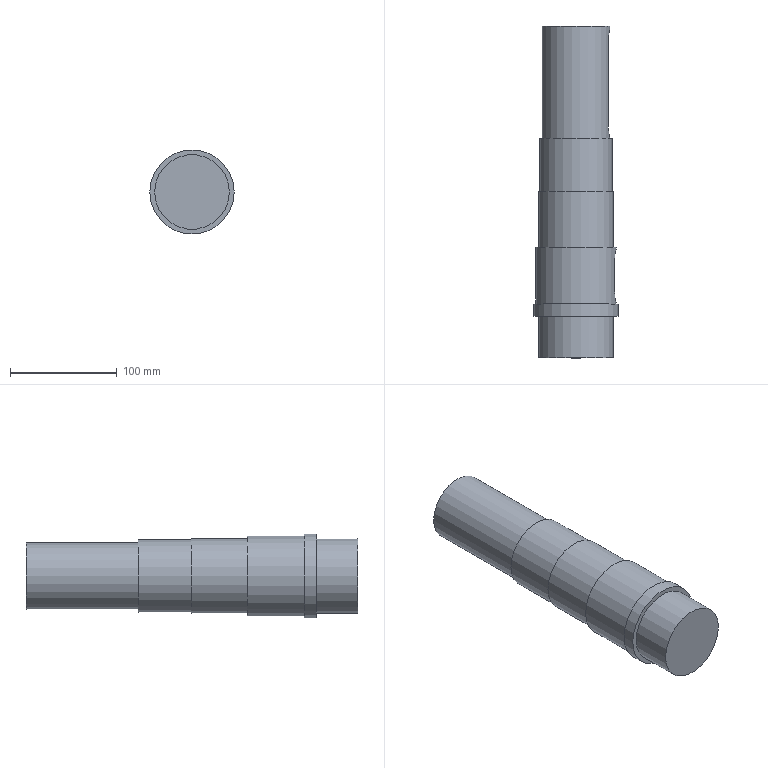Part | NX | features DATUM_CSYS 9, EXTRUDE 8, SKETCH 8, BLEND 2 | 1 solid | 23 faces | box 79 x 311 x 79 mm | volume 1137641 mm3 | plane 13 | cylinder 10 | commonest cylinder face diameters 18 x2 20 x2 70 x2 63 x1 68 x1 75 x1
STEP:
#1=CARTESIAN_POINT('',(35.,0.,0.));
#2=VERTEX_POINT('',#1);
#3=CARTESIAN_POINT('',(0.,0.,0.));
#4=DIRECTION('',(0.,-1.,0.));
#5=DIRECTION('',(1.,0.,0.));
#6=AXIS2_PLACEMENT_3D('',#3,#4,#5);
#7=CIRCLE('',#6,35.);
#8=EDGE_CURVE('',#2,#2,#7,.T.);
#9=ORIENTED_EDGE('',*,*,#8,.T.);
#10=EDGE_LOOP('',(#9));
#11=FACE_BOUND('',#10,.T.);
#12=CARTESIAN_POINT('',(35.,-39.,0.));
#13=VERTEX_POINT('',#12);
#14=CARTESIAN_POINT('',(0.,-39.,0.));
#15=DIRECTION('',(0.,-1.,0.));
#16=DIRECTION('',(1.,0.,0.));
#17=AXIS2_PLACEMENT_3D('',#14,#15,#16);
#18=CIRCLE('',#17,35.);
#19=EDGE_CURVE('',#13,#13,#18,.T.);
#20=ORIENTED_EDGE('',*,*,#19,.F.);
#21=EDGE_LOOP('',(#20));
#22=FACE_BOUND('',#21,.T.);
#23=CARTESIAN_POINT('',(0.,0.,0.));
#24=DIRECTION('',(0.,-1.,0.));
#25=DIRECTION('',(0.,0.,-1.));
#26=AXIS2_PLACEMENT_3D('',#23,#24,#25);
#27=CYLINDRICAL_SURFACE('',#26,35.);
#28=ADVANCED_FACE('',(#11,#22),#27,.T.);
#29=ORIENTED_EDGE('',*,*,#19,.T.);
#30=EDGE_LOOP('',(#29));
#31=FACE_BOUND('',#30,.T.);
#32=CARTESIAN_POINT('',(0.,-39.,0.));
#33=DIRECTION('',(0.,-1.,0.));
#34=DIRECTION('',(0.,0.,-1.));
#35=AXIS2_PLACEMENT_3D('',#32,#33,#34);
#36=PLANE('',#35);
#37=ADVANCED_FACE('',(#31),#36,.T.);
#38=CARTESIAN_POINT('',(39.5,0.,0.));
#39=VERTEX_POINT('',#38);
#40=CARTESIAN_POINT('',(0.,0.,0.));
#41=DIRECTION('',(0.,1.,0.));
#42=DIRECTION('',(1.,0.,0.));
#43=AXIS2_PLACEMENT_3D('',#40,#41,#42);
#44=CIRCLE('',#43,39.5);
#45=EDGE_CURVE('',#39,#39,#44,.T.);
#46=ORIENTED_EDGE('',*,*,#45,.T.);
#47=EDGE_LOOP('',(#46));
#48=FACE_BOUND('',#47,.T.);
#49=CARTESIAN_POINT('',(39.5,11.5,0.));
#50=VERTEX_POINT('',#49);
#51=CARTESIAN_POINT('',(0.,11.5,0.));
#52=DIRECTION('',(0.,1.,0.));
#53=DIRECTION('',(1.,0.,0.));
#54=AXIS2_PLACEMENT_3D('',#51,#52,#53);
#55=CIRCLE('',#54,39.5);
#56=EDGE_CURVE('',#50,#50,#55,.T.);
#57=ORIENTED_EDGE('',*,*,#56,.F.);
#58=EDGE_LOOP('',(#57));
#59=FACE_BOUND('',#58,.T.);
#60=CARTESIAN_POINT('',(0.,0.,0.));
#61=DIRECTION('',(0.,1.,0.));
#62=DIRECTION('',(0.,0.,1.));
#63=AXIS2_PLACEMENT_3D('',#60,#61,#62);
#64=CYLINDRICAL_SURFACE('',#63,39.5);
#65=ADVANCED_FACE('',(#48,#59),#64,.T.);
#66=ORIENTED_EDGE('',*,*,#8,.F.);
#67=EDGE_LOOP('',(#66));
#68=FACE_BOUND('',#67,.T.);
#69=ORIENTED_EDGE('',*,*,#45,.F.);
#70=EDGE_LOOP('',(#69));
#71=FACE_BOUND('',#70,.T.);
#72=CARTESIAN_POINT('',(0.,0.,0.));
#73=DIRECTION('',(0.,1.,0.));
#74=DIRECTION('',(0.,0.,1.));
#75=AXIS2_PLACEMENT_3D('',#72,#73,#74);
#76=PLANE('',#75);
#77=ADVANCED_FACE('',(#68,#71),#76,.F.);
#78=CARTESIAN_POINT('',(37.5,11.5,0.));
#79=VERTEX_POINT('',#78);
#80=CARTESIAN_POINT('',(0.,11.5,0.));
#81=DIRECTION('',(0.,1.,0.));
#82=DIRECTION('',(1.,0.,0.));
#83=AXIS2_PLACEMENT_3D('',#80,#81,#82);
#84=CIRCLE('',#83,37.5);
#85=EDGE_CURVE('',#79,#79,#84,.T.);
#86=ORIENTED_EDGE('',*,*,#85,.F.);
#87=EDGE_LOOP('',(#86));
#88=FACE_BOUND('',#87,.T.);
#89=ORIENTED_EDGE('',*,*,#56,.T.);
#90=EDGE_LOOP('',(#89));
#91=FACE_BOUND('',#90,.T.);
#92=CARTESIAN_POINT('',(0.,11.5,0.));
#93=DIRECTION('',(0.,1.,0.));
#94=DIRECTION('',(0.,0.,1.));
#95=AXIS2_PLACEMENT_3D('',#92,#93,#94);
#96=PLANE('',#95);
#97=ADVANCED_FACE('',(#88,#91),#96,.T.);
#98=CARTESIAN_POINT('',(36.142,23.,-10.));
#99=VERTEX_POINT('',#98);
#100=CARTESIAN_POINT('',(36.142,23.,10.));
#101=VERTEX_POINT('',#100);
#102=CARTESIAN_POINT('',(36.142,23.,-10.));
#103=CARTESIAN_POINT('',(36.142,20.346,-10.));
#104=CARTESIAN_POINT('',(36.649,16.486,-8.359));
#105=CARTESIAN_POINT('',(37.352,13.534,-3.955));
#106=CARTESIAN_POINT('',(37.656,12.461,1.328));
#107=CARTESIAN_POINT('',(36.838,15.18,7.826));
#108=CARTESIAN_POINT('',(36.142,20.346,10.));
#109=CARTESIAN_POINT('',(36.142,23.,10.));
#110=B_SPLINE_CURVE_WITH_KNOTS('',3,(#102,#103,#104,#105,#106,#107,#108,#109),.UNSPECIFIED.,.F.,.F.,(4,1,1,1,1,4),(0.,0.007847,0.01177,0.01569,0.02354,0.03139),.UNSPECIFIED.);
#111=EDGE_CURVE('',#99,#101,#110,.T.);
#112=ORIENTED_EDGE('',*,*,#111,.T.);
#113=CARTESIAN_POINT('',(36.142,53.,10.));
#114=VERTEX_POINT('',#113);
#115=CARTESIAN_POINT('',(36.142,11.5,10.));
#116=DIRECTION('',(0.,1.,0.));
#117=VECTOR('',#116,1000.);
#118=LINE('',#115,#117);
#119=EDGE_CURVE('',#114,#101,#118,.F.);
#120=ORIENTED_EDGE('',*,*,#119,.F.);
#121=CARTESIAN_POINT('',(36.142,53.,-10.));
#122=VERTEX_POINT('',#121);
#123=CARTESIAN_POINT('',(36.142,53.,10.));
#124=CARTESIAN_POINT('',(36.142,55.654,10.));
#125=CARTESIAN_POINT('',(36.649,59.514,8.359));
#126=CARTESIAN_POINT('',(37.352,62.466,3.955));
#127=CARTESIAN_POINT('',(37.656,63.539,-1.328));
#128=CARTESIAN_POINT('',(36.838,60.82,-7.826));
#129=CARTESIAN_POINT('',(36.142,55.654,-10.));
#130=CARTESIAN_POINT('',(36.142,53.,-10.));
#131=B_SPLINE_CURVE_WITH_KNOTS('',3,(#123,#124,#125,#126,#127,#128,#129,#130),.UNSPECIFIED.,.F.,.F.,(4,1,1,1,1,4),(-0.01569,-0.007846,-0.003923,0.000000187,0.007847,0.01569),.UNSPECIFIED.);
#132=EDGE_CURVE('',#114,#122,#131,.T.);
#133=ORIENTED_EDGE('',*,*,#132,.T.);
#134=CARTESIAN_POINT('',(36.142,11.5,-10.));
#135=DIRECTION('',(0.,1.,0.));
#136=VECTOR('',#135,1000.);
#137=LINE('',#134,#136);
#138=EDGE_CURVE('',#99,#122,#137,.T.);
#139=ORIENTED_EDGE('',*,*,#138,.F.);
#140=EDGE_LOOP('',(#112,#120,#133,#139));
#141=FACE_BOUND('',#140,.T.);
#142=ORIENTED_EDGE('',*,*,#85,.T.);
#143=EDGE_LOOP('',(#142));
#144=FACE_BOUND('',#143,.T.);
#145=CARTESIAN_POINT('',(37.5,64.5,0.));
#146=VERTEX_POINT('',#145);
#147=CARTESIAN_POINT('',(0.,64.5,0.));
#148=DIRECTION('',(0.,1.,0.));
#149=DIRECTION('',(1.,0.,0.));
#150=AXIS2_PLACEMENT_3D('',#147,#148,#149);
#151=CIRCLE('',#150,37.5);
#152=EDGE_CURVE('',#146,#146,#151,.T.);
#153=ORIENTED_EDGE('',*,*,#152,.F.);
#154=EDGE_LOOP('',(#153));
#155=FACE_BOUND('',#154,.T.);
#156=CARTESIAN_POINT('',(0.,11.5,0.));
#157=DIRECTION('',(0.,1.,0.));
#158=DIRECTION('',(0.,0.,1.));
#159=AXIS2_PLACEMENT_3D('',#156,#157,#158);
#160=CYLINDRICAL_SURFACE('',#159,37.5);
#161=ADVANCED_FACE('',(#141,#144,#155),#160,.T.);
#162=CARTESIAN_POINT('',(35.,64.5,0.));
#163=VERTEX_POINT('',#162);
#164=CARTESIAN_POINT('',(0.,64.5,0.));
#165=DIRECTION('',(0.,1.,0.));
#166=DIRECTION('',(1.,0.,0.));
#167=AXIS2_PLACEMENT_3D('',#164,#165,#166);
#168=CIRCLE('',#167,35.);
#169=EDGE_CURVE('',#163,#163,#168,.T.);
#170=ORIENTED_EDGE('',*,*,#169,.F.);
#171=EDGE_LOOP('',(#170));
#172=FACE_BOUND('',#171,.T.);
#173=ORIENTED_EDGE('',*,*,#152,.T.);
#174=EDGE_LOOP('',(#173));
#175=FACE_BOUND('',#174,.T.);
#176=CARTESIAN_POINT('',(0.,64.5,0.));
#177=DIRECTION('',(0.,1.,0.));
#178=DIRECTION('',(0.,0.,1.));
#179=AXIS2_PLACEMENT_3D('',#176,#177,#178);
#180=PLANE('',#179);
#181=ADVANCED_FACE('',(#172,#175),#180,.T.);
#182=ORIENTED_EDGE('',*,*,#169,.T.);
#183=EDGE_LOOP('',(#182));
#184=FACE_BOUND('',#183,.T.);
#185=CARTESIAN_POINT('',(35.,117.,0.));
#186=VERTEX_POINT('',#185);
#187=CARTESIAN_POINT('',(0.,117.,0.));
#188=DIRECTION('',(0.,1.,0.));
#189=DIRECTION('',(1.,0.,0.));
#190=AXIS2_PLACEMENT_3D('',#187,#188,#189);
#191=CIRCLE('',#190,35.);
#192=EDGE_CURVE('',#186,#186,#191,.T.);
#193=ORIENTED_EDGE('',*,*,#192,.F.);
#194=EDGE_LOOP('',(#193));
#195=FACE_BOUND('',#194,.T.);
#196=CARTESIAN_POINT('',(0.,64.5,0.));
#197=DIRECTION('',(0.,1.,0.));
#198=DIRECTION('',(0.,0.,1.));
#199=AXIS2_PLACEMENT_3D('',#196,#197,#198);
#200=CYLINDRICAL_SURFACE('',#199,35.);
#201=ADVANCED_FACE('',(#184,#195),#200,.T.);
#202=CARTESIAN_POINT('',(34.,117.,0.));
#203=VERTEX_POINT('',#202);
#204=CARTESIAN_POINT('',(0.,117.,0.));
#205=DIRECTION('',(0.,1.,0.));
#206=DIRECTION('',(1.,0.,0.));
#207=AXIS2_PLACEMENT_3D('',#204,#205,#206);
#208=CIRCLE('',#207,34.);
#209=EDGE_CURVE('',#203,#203,#208,.T.);
#210=ORIENTED_EDGE('',*,*,#209,.F.);
#211=EDGE_LOOP('',(#210));
#212=FACE_BOUND('',#211,.T.);
#213=ORIENTED_EDGE('',*,*,#192,.T.);
#214=EDGE_LOOP('',(#213));
#215=FACE_BOUND('',#214,.T.);
#216=CARTESIAN_POINT('',(0.,117.,0.));
#217=DIRECTION('',(0.,1.,0.));
#218=DIRECTION('',(0.,0.,1.));
#219=AXIS2_PLACEMENT_3D('',#216,#217,#218);
#220=PLANE('',#219);
#221=ADVANCED_FACE('',(#212,#215),#220,.T.);
#222=ORIENTED_EDGE('',*,*,#209,.T.);
#223=EDGE_LOOP('',(#222));
#224=FACE_BOUND('',#223,.T.);
#225=CARTESIAN_POINT('',(34.,167.,0.));
#226=VERTEX_POINT('',#225);
#227=CARTESIAN_POINT('',(0.,167.,0.));
#228=DIRECTION('',(0.,1.,0.));
#229=DIRECTION('',(1.,0.,0.));
#230=AXIS2_PLACEMENT_3D('',#227,#228,#229);
#231=CIRCLE('',#230,34.);
#232=EDGE_CURVE('',#226,#226,#231,.T.);
#233=ORIENTED_EDGE('',*,*,#232,.F.);
#234=EDGE_LOOP('',(#233));
#235=FACE_BOUND('',#234,.T.);
#236=CARTESIAN_POINT('',(0.,117.,0.));
#237=DIRECTION('',(0.,1.,0.));
#238=DIRECTION('',(0.,0.,1.));
#239=AXIS2_PLACEMENT_3D('',#236,#237,#238);
#240=CYLINDRICAL_SURFACE('',#239,34.);
#241=ADVANCED_FACE('',(#224,#235),#240,.T.);
#242=CARTESIAN_POINT('',(31.5,167.,0.));
#243=VERTEX_POINT('',#242);
#244=CARTESIAN_POINT('',(0.,167.,0.));
#245=DIRECTION('',(0.,1.,0.));
#246=DIRECTION('',(1.,0.,0.));
#247=AXIS2_PLACEMENT_3D('',#244,#245,#246);
#248=CIRCLE('',#247,31.5);
#249=EDGE_CURVE('',#243,#243,#248,.T.);
#250=ORIENTED_EDGE('',*,*,#249,.F.);
#251=EDGE_LOOP('',(#250));
#252=FACE_BOUND('',#251,.T.);
#253=ORIENTED_EDGE('',*,*,#232,.T.);
#254=EDGE_LOOP('',(#253));
#255=FACE_BOUND('',#254,.T.);
#256=CARTESIAN_POINT('',(0.,167.,0.));
#257=DIRECTION('',(0.,1.,0.));
#258=DIRECTION('',(0.,0.,1.));
#259=AXIS2_PLACEMENT_3D('',#256,#257,#258);
#260=PLANE('',#259);
#261=ADVANCED_FACE('',(#252,#255),#260,.T.);
#262=CARTESIAN_POINT('',(30.187,177.5,-9.));
#263=VERTEX_POINT('',#262);
#264=CARTESIAN_POINT('',(30.187,177.5,9.));
#265=VERTEX_POINT('',#264);
#266=CARTESIAN_POINT('',(30.187,177.5,-9.));
#267=CARTESIAN_POINT('',(30.187,175.109,-9.));
#268=CARTESIAN_POINT('',(30.678,171.638,-7.521));
#269=CARTESIAN_POINT('',(31.358,168.981,-3.562));
#270=CARTESIAN_POINT('',(31.65,168.014,1.197));
#271=CARTESIAN_POINT('',(30.862,170.463,7.043));
#272=CARTESIAN_POINT('',(30.187,175.11,9.));
#273=CARTESIAN_POINT('',(30.187,177.5,9.));
#274=B_SPLINE_CURVE_WITH_KNOTS('',3,(#266,#267,#268,#269,#270,#271,#272,#273),.UNSPECIFIED.,.F.,.F.,(4,1,1,1,1,4),(0.,0.007067,0.0106,0.01413,0.0212,0.02827),.UNSPECIFIED.);
#275=EDGE_CURVE('',#263,#265,#274,.T.);
#276=ORIENTED_EDGE('',*,*,#275,.T.);
#277=CARTESIAN_POINT('',(30.187,259.5,9.));
#278=VERTEX_POINT('',#277);
#279=CARTESIAN_POINT('',(30.187,167.,9.));
#280=DIRECTION('',(0.,1.,0.));
#281=VECTOR('',#280,1000.);
#282=LINE('',#279,#281);
#283=EDGE_CURVE('',#278,#265,#282,.F.);
#284=ORIENTED_EDGE('',*,*,#283,.F.);
#285=CARTESIAN_POINT('',(30.187,259.5,-9.));
#286=VERTEX_POINT('',#285);
#287=CARTESIAN_POINT('',(30.187,259.5,9.));
#288=CARTESIAN_POINT('',(30.187,261.891,9.));
#289=CARTESIAN_POINT('',(30.678,265.362,7.521));
#290=CARTESIAN_POINT('',(31.358,268.019,3.562));
#291=CARTESIAN_POINT('',(31.65,268.986,-1.197));
#292=CARTESIAN_POINT('',(30.862,266.537,-7.043));
#293=CARTESIAN_POINT('',(30.187,261.89,-9.));
#294=CARTESIAN_POINT('',(30.187,259.5,-9.));
#295=B_SPLINE_CURVE_WITH_KNOTS('',3,(#287,#288,#289,#290,#291,#292,#293,#294),.UNSPECIFIED.,.F.,.F.,(4,1,1,1,1,4),(0.,0.007067,0.0106,0.01413,0.0212,0.02827),.UNSPECIFIED.);
#296=EDGE_CURVE('',#278,#286,#295,.T.);
#297=ORIENTED_EDGE('',*,*,#296,.T.);
#298=CARTESIAN_POINT('',(30.187,167.,-9.));
#299=DIRECTION('',(0.,1.,0.));
#300=VECTOR('',#299,1000.);
#301=LINE('',#298,#300);
#302=EDGE_CURVE('',#263,#286,#301,.T.);
#303=ORIENTED_EDGE('',*,*,#302,.F.);
#304=EDGE_LOOP('',(#276,#284,#297,#303));
#305=FACE_BOUND('',#304,.T.);
#306=ORIENTED_EDGE('',*,*,#249,.T.);
#307=EDGE_LOOP('',(#306));
#308=FACE_BOUND('',#307,.T.);
#309=CARTESIAN_POINT('',(31.5,272.,0.));
#310=VERTEX_POINT('',#309);
#311=CARTESIAN_POINT('',(0.,272.,0.));
#312=DIRECTION('',(0.,1.,0.));
#313=DIRECTION('',(1.,0.,0.));
#314=AXIS2_PLACEMENT_3D('',#311,#312,#313);
#315=CIRCLE('',#314,31.5);
#316=EDGE_CURVE('',#310,#310,#315,.T.);
#317=ORIENTED_EDGE('',*,*,#316,.F.);
#318=EDGE_LOOP('',(#317));
#319=FACE_BOUND('',#318,.T.);
#320=CARTESIAN_POINT('',(0.,167.,0.));
#321=DIRECTION('',(0.,1.,0.));
#322=DIRECTION('',(0.,0.,1.));
#323=AXIS2_PLACEMENT_3D('',#320,#321,#322);
#324=CYLINDRICAL_SURFACE('',#323,31.5);
#325=ADVANCED_FACE('',(#305,#308,#319),#324,.T.);
#326=ORIENTED_EDGE('',*,*,#316,.T.);
#327=EDGE_LOOP('',(#326));
#328=FACE_BOUND('',#327,.T.);
#329=CARTESIAN_POINT('',(0.,272.,0.));
#330=DIRECTION('',(0.,1.,0.));
#331=DIRECTION('',(0.,0.,1.));
#332=AXIS2_PLACEMENT_3D('',#329,#330,#331);
#333=PLANE('',#332);
#334=ADVANCED_FACE('',(#328),#333,.T.);
#335=ORIENTED_EDGE('',*,*,#302,.T.);
#336=CARTESIAN_POINT('',(26.,259.5,-9.));
#337=VERTEX_POINT('',#336);
#338=CARTESIAN_POINT('',(26.,259.5,-9.));
#339=DIRECTION('',(-1.,0.,0.));
#340=VECTOR('',#339,1000.);
#341=LINE('',#338,#340);
#342=EDGE_CURVE('',#286,#337,#341,.T.);
#343=ORIENTED_EDGE('',*,*,#342,.T.);
#344=CARTESIAN_POINT('',(26.,177.5,-9.));
#345=VERTEX_POINT('',#344);
#346=CARTESIAN_POINT('',(26.,168.5,-9.));
#347=DIRECTION('',(0.,1.,0.));
#348=VECTOR('',#347,1000.);
#349=LINE('',#346,#348);
#350=EDGE_CURVE('',#337,#345,#349,.F.);
#351=ORIENTED_EDGE('',*,*,#350,.T.);
#352=CARTESIAN_POINT('',(30.187,177.5,-9.));
#353=DIRECTION('',(-1.,0.,0.));
#354=VECTOR('',#353,1000.);
#355=LINE('',#352,#354);
#356=EDGE_CURVE('',#345,#263,#355,.F.);
#357=ORIENTED_EDGE('',*,*,#356,.T.);
#358=EDGE_LOOP('',(#335,#343,#351,#357));
#359=FACE_BOUND('',#358,.T.);
#360=CARTESIAN_POINT('',(26.,168.5,-9.));
#361=DIRECTION('',(0.,0.,-1.));
#362=DIRECTION('',(0.,1.,0.));
#363=AXIS2_PLACEMENT_3D('',#360,#361,#362);
#364=PLANE('',#363);
#365=ADVANCED_FACE('',(#359),#364,.F.);
#366=CARTESIAN_POINT('',(26.,177.5,9.));
#367=VERTEX_POINT('',#366);
#368=CARTESIAN_POINT('',(26.,259.5,9.));
#369=VERTEX_POINT('',#368);
#370=CARTESIAN_POINT('',(26.,268.5,9.));
#371=DIRECTION('',(0.,-1.,0.));
#372=VECTOR('',#371,1000.);
#373=LINE('',#370,#372);
#374=EDGE_CURVE('',#367,#369,#373,.F.);
#375=ORIENTED_EDGE('',*,*,#374,.T.);
#376=CARTESIAN_POINT('',(30.187,259.5,9.));
#377=DIRECTION('',(-1.,0.,0.));
#378=VECTOR('',#377,1000.);
#379=LINE('',#376,#378);
#380=EDGE_CURVE('',#369,#278,#379,.F.);
#381=ORIENTED_EDGE('',*,*,#380,.T.);
#382=ORIENTED_EDGE('',*,*,#283,.T.);
#383=CARTESIAN_POINT('',(26.,177.5,9.));
#384=DIRECTION('',(-1.,0.,0.));
#385=VECTOR('',#384,1000.);
#386=LINE('',#383,#385);
#387=EDGE_CURVE('',#265,#367,#386,.T.);
#388=ORIENTED_EDGE('',*,*,#387,.T.);
#389=EDGE_LOOP('',(#375,#381,#382,#388));
#390=FACE_BOUND('',#389,.T.);
#391=CARTESIAN_POINT('',(26.,268.5,9.));
#392=DIRECTION('',(0.,0.,1.));
#393=DIRECTION('',(0.,-1.,0.));
#394=AXIS2_PLACEMENT_3D('',#391,#392,#393);
#395=PLANE('',#394);
#396=ADVANCED_FACE('',(#390),#395,.F.);
#397=CARTESIAN_POINT('',(26.,259.5,0.));
#398=DIRECTION('',(1.,0.,0.));
#399=DIRECTION('',(0.,0.,-1.));
#400=AXIS2_PLACEMENT_3D('',#397,#398,#399);
#401=CIRCLE('',#400,9.);
#402=EDGE_CURVE('',#337,#369,#401,.T.);
#403=ORIENTED_EDGE('',*,*,#402,.T.);
#404=ORIENTED_EDGE('',*,*,#374,.F.);
#405=CARTESIAN_POINT('',(26.,177.5,0.));
#406=DIRECTION('',(1.,0.,0.));
#407=DIRECTION('',(0.,0.,-1.));
#408=AXIS2_PLACEMENT_3D('',#405,#406,#407);
#409=CIRCLE('',#408,9.);
#410=EDGE_CURVE('',#367,#345,#409,.T.);
#411=ORIENTED_EDGE('',*,*,#410,.T.);
#412=ORIENTED_EDGE('',*,*,#350,.F.);
#413=EDGE_LOOP('',(#403,#404,#411,#412));
#414=FACE_BOUND('',#413,.T.);
#415=CARTESIAN_POINT('',(26.,0.,0.));
#416=DIRECTION('',(1.,0.,0.));
#417=DIRECTION('',(0.,0.,-1.));
#418=AXIS2_PLACEMENT_3D('',#415,#416,#417);
#419=PLANE('',#418);
#420=ADVANCED_FACE('',(#414),#419,.T.);
#421=ORIENTED_EDGE('',*,*,#342,.F.);
#422=ORIENTED_EDGE('',*,*,#296,.F.);
#423=ORIENTED_EDGE('',*,*,#380,.F.);
#424=ORIENTED_EDGE('',*,*,#402,.F.);
#425=EDGE_LOOP('',(#421,#422,#423,#424));
#426=FACE_BOUND('',#425,.T.);
#427=CARTESIAN_POINT('',(26.,259.5,0.));
#428=DIRECTION('',(1.,0.,0.));
#429=DIRECTION('',(0.,0.,-1.));
#430=AXIS2_PLACEMENT_3D('',#427,#428,#429);
#431=CYLINDRICAL_SURFACE('',#430,9.);
#432=ADVANCED_FACE('',(#426),#431,.F.);
#433=ORIENTED_EDGE('',*,*,#387,.F.);
#434=ORIENTED_EDGE('',*,*,#275,.F.);
#435=ORIENTED_EDGE('',*,*,#356,.F.);
#436=ORIENTED_EDGE('',*,*,#410,.F.);
#437=EDGE_LOOP('',(#433,#434,#435,#436));
#438=FACE_BOUND('',#437,.T.);
#439=CARTESIAN_POINT('',(26.,177.5,0.));
#440=DIRECTION('',(1.,0.,0.));
#441=DIRECTION('',(0.,0.,-1.));
#442=AXIS2_PLACEMENT_3D('',#439,#440,#441);
#443=CYLINDRICAL_SURFACE('',#442,9.);
#444=ADVANCED_FACE('',(#438),#443,.F.);
#445=ORIENTED_EDGE('',*,*,#138,.T.);
#446=CARTESIAN_POINT('',(31.5,53.,-10.));
#447=VERTEX_POINT('',#446);
#448=CARTESIAN_POINT('',(31.5,53.,-10.));
#449=DIRECTION('',(-1.,0.,0.));
#450=VECTOR('',#449,1000.);
#451=LINE('',#448,#450);
#452=EDGE_CURVE('',#122,#447,#451,.T.);
#453=ORIENTED_EDGE('',*,*,#452,.T.);
#454=CARTESIAN_POINT('',(31.5,23.,-10.));
#455=VERTEX_POINT('',#454);
#456=CARTESIAN_POINT('',(31.5,13.,-10.));
#457=DIRECTION('',(0.,1.,0.));
#458=VECTOR('',#457,1000.);
#459=LINE('',#456,#458);
#460=EDGE_CURVE('',#447,#455,#459,.F.);
#461=ORIENTED_EDGE('',*,*,#460,.T.);
#462=CARTESIAN_POINT('',(36.142,23.,-10.));
#463=DIRECTION('',(-1.,0.,0.));
#464=VECTOR('',#463,1000.);
#465=LINE('',#462,#464);
#466=EDGE_CURVE('',#455,#99,#465,.F.);
#467=ORIENTED_EDGE('',*,*,#466,.T.);
#468=EDGE_LOOP('',(#445,#453,#461,#467));
#469=FACE_BOUND('',#468,.T.);
#470=CARTESIAN_POINT('',(31.5,13.,-10.));
#471=DIRECTION('',(0.,0.,-1.));
#472=DIRECTION('',(0.,1.,0.));
#473=AXIS2_PLACEMENT_3D('',#470,#471,#472);
#474=PLANE('',#473);
#475=ADVANCED_FACE('',(#469),#474,.F.);
#476=ORIENTED_EDGE('',*,*,#119,.T.);
#477=CARTESIAN_POINT('',(31.5,23.,10.));
#478=VERTEX_POINT('',#477);
#479=CARTESIAN_POINT('',(31.5,23.,10.));
#480=DIRECTION('',(-1.,0.,0.));
#481=VECTOR('',#480,1000.);
#482=LINE('',#479,#481);
#483=EDGE_CURVE('',#101,#478,#482,.T.);
#484=ORIENTED_EDGE('',*,*,#483,.T.);
#485=CARTESIAN_POINT('',(31.5,53.,10.));
#486=VERTEX_POINT('',#485);
#487=CARTESIAN_POINT('',(31.5,63.,10.));
#488=DIRECTION('',(0.,-1.,0.));
#489=VECTOR('',#488,1000.);
#490=LINE('',#487,#489);
#491=EDGE_CURVE('',#478,#486,#490,.F.);
#492=ORIENTED_EDGE('',*,*,#491,.T.);
#493=CARTESIAN_POINT('',(36.142,53.,10.));
#494=DIRECTION('',(-1.,0.,0.));
#495=VECTOR('',#494,1000.);
#496=LINE('',#493,#495);
#497=EDGE_CURVE('',#486,#114,#496,.F.);
#498=ORIENTED_EDGE('',*,*,#497,.T.);
#499=EDGE_LOOP('',(#476,#484,#492,#498));
#500=FACE_BOUND('',#499,.T.);
#501=CARTESIAN_POINT('',(31.5,63.,10.));
#502=DIRECTION('',(0.,0.,1.));
#503=DIRECTION('',(0.,-1.,0.));
#504=AXIS2_PLACEMENT_3D('',#501,#502,#503);
#505=PLANE('',#504);
#506=ADVANCED_FACE('',(#500),#505,.F.);
#507=CARTESIAN_POINT('',(31.5,23.,0.));
#508=DIRECTION('',(1.,0.,0.));
#509=DIRECTION('',(0.,0.,-1.));
#510=AXIS2_PLACEMENT_3D('',#507,#508,#509);
#511=CIRCLE('',#510,10.);
#512=EDGE_CURVE('',#478,#455,#511,.T.);
#513=ORIENTED_EDGE('',*,*,#512,.T.);
#514=ORIENTED_EDGE('',*,*,#460,.F.);
#515=CARTESIAN_POINT('',(31.5,53.,0.));
#516=DIRECTION('',(1.,0.,0.));
#517=DIRECTION('',(0.,0.,-1.));
#518=AXIS2_PLACEMENT_3D('',#515,#516,#517);
#519=CIRCLE('',#518,10.);
#520=EDGE_CURVE('',#447,#486,#519,.T.);
#521=ORIENTED_EDGE('',*,*,#520,.T.);
#522=ORIENTED_EDGE('',*,*,#491,.F.);
#523=EDGE_LOOP('',(#513,#514,#521,#522));
#524=FACE_BOUND('',#523,.T.);
#525=CARTESIAN_POINT('',(31.5,0.,0.));
#526=DIRECTION('',(1.,0.,0.));
#527=DIRECTION('',(0.,0.,-1.));
#528=AXIS2_PLACEMENT_3D('',#525,#526,#527);
#529=PLANE('',#528);
#530=ADVANCED_FACE('',(#524),#529,.T.);
#531=ORIENTED_EDGE('',*,*,#520,.F.);
#532=ORIENTED_EDGE('',*,*,#452,.F.);
#533=ORIENTED_EDGE('',*,*,#132,.F.);
#534=ORIENTED_EDGE('',*,*,#497,.F.);
#535=EDGE_LOOP('',(#531,#532,#533,#534));
#536=FACE_BOUND('',#535,.T.);
#537=CARTESIAN_POINT('',(31.5,53.,0.));
#538=DIRECTION('',(1.,0.,0.));
#539=DIRECTION('',(0.,0.,-1.));
#540=AXIS2_PLACEMENT_3D('',#537,#538,#539);
#541=CYLINDRICAL_SURFACE('',#540,10.);
#542=ADVANCED_FACE('',(#536),#541,.F.);
#543=ORIENTED_EDGE('',*,*,#483,.F.);
#544=ORIENTED_EDGE('',*,*,#111,.F.);
#545=ORIENTED_EDGE('',*,*,#466,.F.);
#546=ORIENTED_EDGE('',*,*,#512,.F.);
#547=EDGE_LOOP('',(#543,#544,#545,#546));
#548=FACE_BOUND('',#547,.T.);
#549=CARTESIAN_POINT('',(31.5,23.,0.));
#550=DIRECTION('',(1.,0.,0.));
#551=DIRECTION('',(0.,0.,-1.));
#552=AXIS2_PLACEMENT_3D('',#549,#550,#551);
#553=CYLINDRICAL_SURFACE('',#552,10.);
#554=ADVANCED_FACE('',(#548),#553,.F.);
#555=CLOSED_SHELL('',(#28,#37,#65,#77,#97,#161,#181,#201,#221,#241,#261,#325,#334,#365,#396,#420,#432,#444,#475,#506,#530,#542,#554));
#556=MANIFOLD_SOLID_BREP('',#555);
#557=(LENGTH_UNIT()NAMED_UNIT(*)SI_UNIT(.MILLI.,.METRE.));
#558=UNCERTAINTY_MEASURE_WITH_UNIT(LENGTH_MEASURE(0.0508),#557,'','');
#559=(NAMED_UNIT(*)PLANE_ANGLE_UNIT()SI_UNIT($,.RADIAN.));
#560=(NAMED_UNIT(*)SI_UNIT($,.STERADIAN.)SOLID_ANGLE_UNIT());
#561=(GEOMETRIC_REPRESENTATION_CONTEXT(3)GLOBAL_UNCERTAINTY_ASSIGNED_CONTEXT((#558))GLOBAL_UNIT_ASSIGNED_CONTEXT((#557,#559,#560))REPRESENTATION_CONTEXT('',''));
#562=ADVANCED_BREP_SHAPE_REPRESENTATION('',(#556),#561);